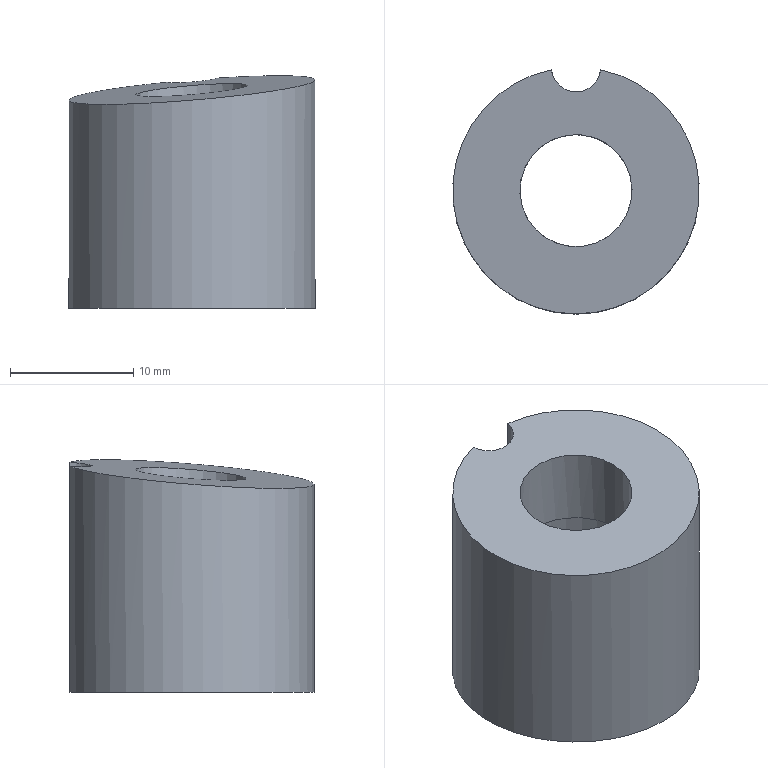Part | NX | features EKSD 20-20-10.10 2 | 1 solid | 7 faces | box 20 x 19.8 x 18.863 mm | volume 3583 mm3 | cylinder 4 | plane 3 | commonest cylinder face diameters 4 x1 9.1 x1 12.6 x1 20 x1
STEP:
#1=CARTESIAN_POINT('',(656.593,-7.961,-27.));
#2=VERTEX_POINT('',#1);
#3=CARTESIAN_POINT('',(660.573,-7.961,-27.));
#4=VERTEX_POINT('',#3);
#5=CARTESIAN_POINT('',(658.583,-7.761,-27.));
#6=DIRECTION('',(0.,0.,1.));
#7=DIRECTION('',(1.,0.,0.));
#8=AXIS2_PLACEMENT_3D('',#5,#6,#7);
#9=CIRCLE('',#8,2.);
#10=EDGE_CURVE('',#2,#4,#9,.T.);
#11=ORIENTED_EDGE('',*,*,#10,.T.);
#12=CARTESIAN_POINT('',(658.583,-17.761,-27.));
#13=DIRECTION('',(0.,0.,1.));
#14=DIRECTION('',(1.,0.,0.));
#15=AXIS2_PLACEMENT_3D('',#12,#13,#14);
#16=CIRCLE('',#15,10.);
#17=EDGE_CURVE('',#2,#4,#16,.T.);
#18=ORIENTED_EDGE('',*,*,#17,.F.);
#19=EDGE_LOOP('',(#11,#18));
#20=FACE_BOUND('',#19,.T.);
#21=CARTESIAN_POINT('',(652.283,-17.761,-27.));
#22=VERTEX_POINT('',#21);
#23=CARTESIAN_POINT('',(658.583,-17.761,-27.));
#24=DIRECTION('',(0.,0.,-1.));
#25=DIRECTION('',(-1.,0.,0.));
#26=AXIS2_PLACEMENT_3D('',#23,#24,#25);
#27=CIRCLE('',#26,6.3);
#28=EDGE_CURVE('',#22,#22,#27,.T.);
#29=ORIENTED_EDGE('',*,*,#28,.F.);
#30=EDGE_LOOP('',(#29));
#31=FACE_BOUND('',#30,.T.);
#32=CARTESIAN_POINT('',(658.583,-17.761,-27.));
#33=DIRECTION('',(0.,0.,-1.));
#34=DIRECTION('',(-1.,0.,0.));
#35=AXIS2_PLACEMENT_3D('',#32,#33,#34);
#36=PLANE('',#35);
#37=ADVANCED_FACE('',(#20,#31),#36,.T.);
#38=CARTESIAN_POINT('',(660.573,-7.961,-8.334));
#39=VERTEX_POINT('',#38);
#40=CARTESIAN_POINT('',(656.593,-7.961,-8.662));
#41=VERTEX_POINT('',#40);
#42=CARTESIAN_POINT('',(658.583,-7.761,-8.482));
#43=DIRECTION('',(0.08207,0.08131,-0.9933));
#44=DIRECTION('',(-0.7057,-0.6991,-0.1155));
#45=AXIS2_PLACEMENT_3D('',#42,#43,#44);
#46=ELLIPSE('',#45,2.013,2.);
#47=EDGE_CURVE('',#39,#41,#46,.T.);
#48=ORIENTED_EDGE('',*,*,#47,.T.);
#49=CARTESIAN_POINT('',(658.583,-17.761,-9.3));
#50=DIRECTION('',(0.08207,0.08131,-0.9933));
#51=DIRECTION('',(-0.7057,-0.6991,-0.1155));
#52=AXIS2_PLACEMENT_3D('',#49,#50,#51);
#53=ELLIPSE('',#52,10.067,10.);
#54=EDGE_CURVE('',#39,#41,#53,.T.);
#55=ORIENTED_EDGE('',*,*,#54,.F.);
#56=EDGE_LOOP('',(#48,#55));
#57=FACE_BOUND('',#56,.T.);
#58=CARTESIAN_POINT('',(655.35,-20.963,-9.829));
#59=VERTEX_POINT('',#58);
#60=CARTESIAN_POINT('',(658.583,-17.761,-9.3));
#61=DIRECTION('',(0.08207,0.08131,-0.9933));
#62=DIRECTION('',(-0.7057,-0.6991,-0.1155));
#63=AXIS2_PLACEMENT_3D('',#60,#61,#62);
#64=ELLIPSE('',#63,4.581,4.55);
#65=EDGE_CURVE('',#59,#59,#64,.F.);
#66=ORIENTED_EDGE('',*,*,#65,.F.);
#67=EDGE_LOOP('',(#66));
#68=FACE_BOUND('',#67,.T.);
#69=CARTESIAN_POINT('',(770.198,-94.894,-6.392));
#70=DIRECTION('',(0.08207,0.08131,-0.9933));
#71=DIRECTION('',(0.9966,-0.01117,0.08143));
#72=AXIS2_PLACEMENT_3D('',#69,#70,#71);
#73=PLANE('',#72);
#74=ADVANCED_FACE('',(#57,#68),#73,.F.);
#75=CARTESIAN_POINT('',(660.573,-7.961,-17.));
#76=DIRECTION('',(0.,0.,-1.));
#77=VECTOR('',#76,1000.);
#78=LINE('',#75,#77);
#79=EDGE_CURVE('',#39,#4,#78,.T.);
#80=ORIENTED_EDGE('',*,*,#79,.F.);
#81=ORIENTED_EDGE('',*,*,#54,.T.);
#82=CARTESIAN_POINT('',(656.593,-7.961,-17.));
#83=DIRECTION('',(0.,0.,-1.));
#84=VECTOR('',#83,1000.);
#85=LINE('',#82,#84);
#86=EDGE_CURVE('',#2,#41,#85,.F.);
#87=ORIENTED_EDGE('',*,*,#86,.F.);
#88=ORIENTED_EDGE('',*,*,#17,.T.);
#89=EDGE_LOOP('',(#80,#81,#87,#88));
#90=FACE_BOUND('',#89,.T.);
#91=CARTESIAN_POINT('',(658.583,-17.761,-7.));
#92=DIRECTION('',(0.,0.,-1.));
#93=DIRECTION('',(-1.,0.,0.));
#94=AXIS2_PLACEMENT_3D('',#91,#92,#93);
#95=CYLINDRICAL_SURFACE('',#94,10.);
#96=ADVANCED_FACE('',(#90),#95,.T.);
#97=CARTESIAN_POINT('',(663.133,-17.761,-15.));
#98=VERTEX_POINT('',#97);
#99=CARTESIAN_POINT('',(658.583,-17.761,-15.));
#100=DIRECTION('',(0.,0.,1.));
#101=DIRECTION('',(1.,0.,0.));
#102=AXIS2_PLACEMENT_3D('',#99,#100,#101);
#103=CIRCLE('',#102,4.55);
#104=EDGE_CURVE('',#98,#98,#103,.F.);
#105=ORIENTED_EDGE('',*,*,#104,.T.);
#106=EDGE_LOOP('',(#105));
#107=FACE_BOUND('',#106,.T.);
#108=ORIENTED_EDGE('',*,*,#65,.T.);
#109=EDGE_LOOP('',(#108));
#110=FACE_BOUND('',#109,.T.);
#111=CARTESIAN_POINT('',(658.583,-17.761,-6.));
#112=DIRECTION('',(0.,0.,-1.));
#113=DIRECTION('',(-1.,0.,0.));
#114=AXIS2_PLACEMENT_3D('',#111,#112,#113);
#115=CYLINDRICAL_SURFACE('',#114,4.55);
#116=ADVANCED_FACE('',(#107,#110),#115,.F.);
#117=CARTESIAN_POINT('',(652.283,-17.761,-15.));
#118=VERTEX_POINT('',#117);
#119=CARTESIAN_POINT('',(658.583,-17.761,-15.));
#120=DIRECTION('',(0.,0.,-1.));
#121=DIRECTION('',(-1.,0.,0.));
#122=AXIS2_PLACEMENT_3D('',#119,#120,#121);
#123=CIRCLE('',#122,6.3);
#124=EDGE_CURVE('',#118,#118,#123,.T.);
#125=ORIENTED_EDGE('',*,*,#124,.T.);
#126=EDGE_LOOP('',(#125));
#127=FACE_BOUND('',#126,.T.);
#128=ORIENTED_EDGE('',*,*,#104,.F.);
#129=EDGE_LOOP('',(#128));
#130=FACE_BOUND('',#129,.T.);
#131=CARTESIAN_POINT('',(658.583,-17.761,-15.));
#132=DIRECTION('',(0.,0.,1.));
#133=DIRECTION('',(1.,0.,0.));
#134=AXIS2_PLACEMENT_3D('',#131,#132,#133);
#135=PLANE('',#134);
#136=ADVANCED_FACE('',(#127,#130),#135,.F.);
#137=ORIENTED_EDGE('',*,*,#28,.T.);
#138=EDGE_LOOP('',(#137));
#139=FACE_BOUND('',#138,.T.);
#140=ORIENTED_EDGE('',*,*,#124,.F.);
#141=EDGE_LOOP('',(#140));
#142=FACE_BOUND('',#141,.T.);
#143=CARTESIAN_POINT('',(658.583,-17.761,-15.));
#144=DIRECTION('',(0.,0.,-1.));
#145=DIRECTION('',(-1.,0.,0.));
#146=AXIS2_PLACEMENT_3D('',#143,#144,#145);
#147=CYLINDRICAL_SURFACE('',#146,6.3);
#148=ADVANCED_FACE('',(#139,#142),#147,.F.);
#149=ORIENTED_EDGE('',*,*,#79,.T.);
#150=ORIENTED_EDGE('',*,*,#10,.F.);
#151=ORIENTED_EDGE('',*,*,#86,.T.);
#152=ORIENTED_EDGE('',*,*,#47,.F.);
#153=EDGE_LOOP('',(#149,#150,#151,#152));
#154=FACE_BOUND('',#153,.T.);
#155=CARTESIAN_POINT('',(658.583,-7.761,-7.));
#156=DIRECTION('',(0.,0.,-1.));
#157=DIRECTION('',(-1.,0.,0.));
#158=AXIS2_PLACEMENT_3D('',#155,#156,#157);
#159=CYLINDRICAL_SURFACE('',#158,2.);
#160=ADVANCED_FACE('',(#154),#159,.F.);
#161=CLOSED_SHELL('',(#37,#74,#96,#116,#136,#148,#160));
#162=MANIFOLD_SOLID_BREP('',#161);
#163=(LENGTH_UNIT()NAMED_UNIT(*)SI_UNIT(.MILLI.,.METRE.));
#164=UNCERTAINTY_MEASURE_WITH_UNIT(LENGTH_MEASURE(0.00001),#163,'','');
#165=(NAMED_UNIT(*)PLANE_ANGLE_UNIT()SI_UNIT($,.RADIAN.));
#166=(NAMED_UNIT(*)SI_UNIT($,.STERADIAN.)SOLID_ANGLE_UNIT());
#167=(GEOMETRIC_REPRESENTATION_CONTEXT(3)GLOBAL_UNCERTAINTY_ASSIGNED_CONTEXT((#164))GLOBAL_UNIT_ASSIGNED_CONTEXT((#163,#165,#166))REPRESENTATION_CONTEXT('',''));
#168=ADVANCED_BREP_SHAPE_REPRESENTATION('',(#162),#167);